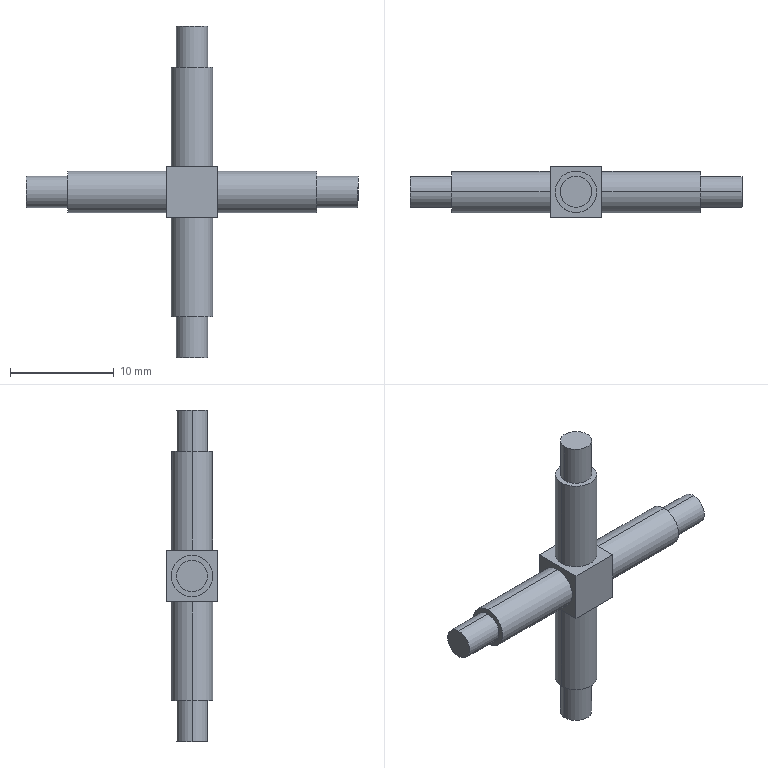Part | SolidWorks | features ICE 4, MirrorPattern 4, Extrusion 1 | 1 solid | 30 faces | box 32 x 5 x 32 mm | volume 715.619 mm3 | cylinder 16 | plane 14 | commonest cylinder face diameters 3 x8 4 x8
STEP:
#1=CARTESIAN_POINT('',(-16.194,28.299,4.));
#2=VERTEX_POINT('',#1);
#3=CARTESIAN_POINT('',(-16.194,28.299,1.));
#4=VERTEX_POINT('',#3);
#5=CARTESIAN_POINT('',(-16.194,28.299,2.5));
#6=DIRECTION('',(-1.,0.,0.));
#7=DIRECTION('',(0.,0.,1.));
#8=AXIS2_PLACEMENT_3D('',#5,#6,#7);
#9=CIRCLE('',#8,1.5);
#10=EDGE_CURVE('',#2,#4,#9,.T.);
#11=ORIENTED_EDGE('',*,*,#10,.F.);
#12=CARTESIAN_POINT('',(-12.194,28.299,4.));
#13=VERTEX_POINT('',#12);
#14=CARTESIAN_POINT('',(-16.194,28.299,4.));
#15=DIRECTION('',(1.,0.,0.));
#16=VECTOR('',#15,1000.);
#17=LINE('',#14,#16);
#18=EDGE_CURVE('',#2,#13,#17,.T.);
#19=ORIENTED_EDGE('',*,*,#18,.T.);
#20=CARTESIAN_POINT('',(-12.194,28.299,1.));
#21=VERTEX_POINT('',#20);
#22=CARTESIAN_POINT('',(-12.194,28.299,2.5));
#23=DIRECTION('',(-1.,0.,0.));
#24=DIRECTION('',(0.,0.,1.));
#25=AXIS2_PLACEMENT_3D('',#22,#23,#24);
#26=CIRCLE('',#25,1.5);
#27=EDGE_CURVE('',#13,#21,#26,.T.);
#28=ORIENTED_EDGE('',*,*,#27,.T.);
#29=CARTESIAN_POINT('',(-16.194,28.299,1.));
#30=DIRECTION('',(1.,0.,0.));
#31=VECTOR('',#30,1000.);
#32=LINE('',#29,#31);
#33=EDGE_CURVE('',#4,#21,#32,.T.);
#34=ORIENTED_EDGE('',*,*,#33,.F.);
#35=EDGE_LOOP('',(#11,#19,#28,#34));
#36=FACE_OUTER_BOUND('',#35,.T.);
#37=CARTESIAN_POINT('',(-16.194,28.299,2.5));
#38=DIRECTION('',(1.,0.,0.));
#39=DIRECTION('',(0.,0.,-1.));
#40=AXIS2_PLACEMENT_3D('',#37,#38,#39);
#41=CYLINDRICAL_SURFACE('',#40,1.5);
#42=ADVANCED_FACE('',(#36),#41,.T.);
#43=CARTESIAN_POINT('',(-40.194,28.299,4.));
#44=VERTEX_POINT('',#43);
#45=CARTESIAN_POINT('',(-40.194,28.299,1.));
#46=VERTEX_POINT('',#45);
#47=CARTESIAN_POINT('',(-40.194,28.299,2.5));
#48=DIRECTION('',(-1.,0.,0.));
#49=DIRECTION('',(0.,0.,1.));
#50=AXIS2_PLACEMENT_3D('',#47,#48,#49);
#51=CIRCLE('',#50,1.5);
#52=EDGE_CURVE('',#44,#46,#51,.T.);
#53=ORIENTED_EDGE('',*,*,#52,.T.);
#54=CARTESIAN_POINT('',(-44.194,28.299,1.));
#55=VERTEX_POINT('',#54);
#56=CARTESIAN_POINT('',(-40.194,28.299,1.));
#57=DIRECTION('',(-1.,0.,0.));
#58=VECTOR('',#57,1000.);
#59=LINE('',#56,#58);
#60=EDGE_CURVE('',#46,#55,#59,.T.);
#61=ORIENTED_EDGE('',*,*,#60,.T.);
#62=CARTESIAN_POINT('',(-44.194,28.299,4.));
#63=VERTEX_POINT('',#62);
#64=CARTESIAN_POINT('',(-44.194,28.299,2.5));
#65=DIRECTION('',(-1.,0.,0.));
#66=DIRECTION('',(0.,0.,1.));
#67=AXIS2_PLACEMENT_3D('',#64,#65,#66);
#68=CIRCLE('',#67,1.5);
#69=EDGE_CURVE('',#63,#55,#68,.T.);
#70=ORIENTED_EDGE('',*,*,#69,.F.);
#71=CARTESIAN_POINT('',(-40.194,28.299,4.));
#72=DIRECTION('',(-1.,0.,0.));
#73=VECTOR('',#72,1000.);
#74=LINE('',#71,#73);
#75=EDGE_CURVE('',#44,#63,#74,.T.);
#76=ORIENTED_EDGE('',*,*,#75,.F.);
#77=EDGE_LOOP('',(#53,#61,#70,#76));
#78=FACE_OUTER_BOUND('',#77,.T.);
#79=CARTESIAN_POINT('',(-40.194,28.299,2.5));
#80=DIRECTION('',(-1.,0.,0.));
#81=DIRECTION('',(0.,0.,1.));
#82=AXIS2_PLACEMENT_3D('',#79,#80,#81);
#83=CYLINDRICAL_SURFACE('',#82,1.5);
#84=ADVANCED_FACE('',(#78),#83,.T.);
#85=CARTESIAN_POINT('',(-26.694,28.299,-9.5));
#86=VERTEX_POINT('',#85);
#87=CARTESIAN_POINT('',(-29.694,28.299,-9.5));
#88=VERTEX_POINT('',#87);
#89=CARTESIAN_POINT('',(-28.194,28.299,-9.5));
#90=DIRECTION('',(0.,0.,1.));
#91=DIRECTION('',(1.,0.,0.));
#92=AXIS2_PLACEMENT_3D('',#89,#90,#91);
#93=CIRCLE('',#92,1.5);
#94=EDGE_CURVE('',#86,#88,#93,.T.);
#95=ORIENTED_EDGE('',*,*,#94,.F.);
#96=CARTESIAN_POINT('',(-26.694,28.299,-13.5));
#97=VERTEX_POINT('',#96);
#98=CARTESIAN_POINT('',(-26.694,28.299,-9.5));
#99=DIRECTION('',(0.,0.,-1.));
#100=VECTOR('',#99,1000.);
#101=LINE('',#98,#100);
#102=EDGE_CURVE('',#86,#97,#101,.T.);
#103=ORIENTED_EDGE('',*,*,#102,.T.);
#104=CARTESIAN_POINT('',(-29.694,28.299,-13.5));
#105=VERTEX_POINT('',#104);
#106=CARTESIAN_POINT('',(-28.194,28.299,-13.5));
#107=DIRECTION('',(0.,0.,1.));
#108=DIRECTION('',(1.,0.,0.));
#109=AXIS2_PLACEMENT_3D('',#106,#107,#108);
#110=CIRCLE('',#109,1.5);
#111=EDGE_CURVE('',#97,#105,#110,.T.);
#112=ORIENTED_EDGE('',*,*,#111,.T.);
#113=CARTESIAN_POINT('',(-29.694,28.299,-9.5));
#114=DIRECTION('',(0.,0.,-1.));
#115=VECTOR('',#114,1000.);
#116=LINE('',#113,#115);
#117=EDGE_CURVE('',#88,#105,#116,.T.);
#118=ORIENTED_EDGE('',*,*,#117,.F.);
#119=EDGE_LOOP('',(#95,#103,#112,#118));
#120=FACE_OUTER_BOUND('',#119,.T.);
#121=CARTESIAN_POINT('',(-28.194,28.299,-9.5));
#122=DIRECTION('',(0.,0.,-1.));
#123=DIRECTION('',(-1.,0.,0.));
#124=AXIS2_PLACEMENT_3D('',#121,#122,#123);
#125=CYLINDRICAL_SURFACE('',#124,1.5);
#126=ADVANCED_FACE('',(#120),#125,.T.);
#127=CARTESIAN_POINT('',(-26.694,28.299,14.5));
#128=VERTEX_POINT('',#127);
#129=CARTESIAN_POINT('',(-29.694,28.299,14.5));
#130=VERTEX_POINT('',#129);
#131=CARTESIAN_POINT('',(-28.194,28.299,14.5));
#132=DIRECTION('',(0.,0.,1.));
#133=DIRECTION('',(1.,0.,0.));
#134=AXIS2_PLACEMENT_3D('',#131,#132,#133);
#135=CIRCLE('',#134,1.5);
#136=EDGE_CURVE('',#128,#130,#135,.T.);
#137=ORIENTED_EDGE('',*,*,#136,.T.);
#138=CARTESIAN_POINT('',(-29.694,28.299,18.5));
#139=VERTEX_POINT('',#138);
#140=CARTESIAN_POINT('',(-29.694,28.299,14.5));
#141=DIRECTION('',(0.,0.,1.));
#142=VECTOR('',#141,1000.);
#143=LINE('',#140,#142);
#144=EDGE_CURVE('',#130,#139,#143,.T.);
#145=ORIENTED_EDGE('',*,*,#144,.T.);
#146=CARTESIAN_POINT('',(-26.694,28.299,18.5));
#147=VERTEX_POINT('',#146);
#148=CARTESIAN_POINT('',(-28.194,28.299,18.5));
#149=DIRECTION('',(0.,0.,1.));
#150=DIRECTION('',(1.,0.,0.));
#151=AXIS2_PLACEMENT_3D('',#148,#149,#150);
#152=CIRCLE('',#151,1.5);
#153=EDGE_CURVE('',#147,#139,#152,.T.);
#154=ORIENTED_EDGE('',*,*,#153,.F.);
#155=CARTESIAN_POINT('',(-26.694,28.299,14.5));
#156=DIRECTION('',(0.,0.,1.));
#157=VECTOR('',#156,1000.);
#158=LINE('',#155,#157);
#159=EDGE_CURVE('',#128,#147,#158,.T.);
#160=ORIENTED_EDGE('',*,*,#159,.F.);
#161=EDGE_LOOP('',(#137,#145,#154,#160));
#162=FACE_OUTER_BOUND('',#161,.T.);
#163=CARTESIAN_POINT('',(-28.194,28.299,14.5));
#164=DIRECTION('',(0.,0.,1.));
#165=DIRECTION('',(1.,0.,0.));
#166=AXIS2_PLACEMENT_3D('',#163,#164,#165);
#167=CYLINDRICAL_SURFACE('',#166,1.5);
#168=ADVANCED_FACE('',(#162),#167,.T.);
#169=CARTESIAN_POINT('',(-26.194,28.299,14.5));
#170=VERTEX_POINT('',#169);
#171=CARTESIAN_POINT('',(-30.194,28.299,14.5));
#172=VERTEX_POINT('',#171);
#173=CARTESIAN_POINT('',(-28.194,28.299,14.5));
#174=DIRECTION('',(0.,0.,1.));
#175=DIRECTION('',(1.,0.,0.));
#176=AXIS2_PLACEMENT_3D('',#173,#174,#175);
#177=CIRCLE('',#176,2.);
#178=EDGE_CURVE('',#170,#172,#177,.T.);
#179=ORIENTED_EDGE('',*,*,#178,.F.);
#180=CARTESIAN_POINT('',(-26.194,28.299,5.));
#181=VERTEX_POINT('',#180);
#182=CARTESIAN_POINT('',(-26.194,28.299,18.5));
#183=DIRECTION('',(0.,0.,-1.));
#184=VECTOR('',#183,1000.);
#185=LINE('',#182,#184);
#186=EDGE_CURVE('',#170,#181,#185,.T.);
#187=ORIENTED_EDGE('',*,*,#186,.T.);
#188=CARTESIAN_POINT('',(-30.194,28.299,5.));
#189=VERTEX_POINT('',#188);
#190=CARTESIAN_POINT('',(-28.194,28.299,5.));
#191=DIRECTION('',(0.,0.,1.));
#192=DIRECTION('',(1.,0.,0.));
#193=AXIS2_PLACEMENT_3D('',#190,#191,#192);
#194=CIRCLE('',#193,2.);
#195=EDGE_CURVE('',#181,#189,#194,.T.);
#196=ORIENTED_EDGE('',*,*,#195,.T.);
#197=CARTESIAN_POINT('',(-30.194,28.299,18.5));
#198=DIRECTION('',(0.,0.,-1.));
#199=VECTOR('',#198,1000.);
#200=LINE('',#197,#199);
#201=EDGE_CURVE('',#172,#189,#200,.T.);
#202=ORIENTED_EDGE('',*,*,#201,.F.);
#203=EDGE_LOOP('',(#179,#187,#196,#202));
#204=FACE_OUTER_BOUND('',#203,.T.);
#205=CARTESIAN_POINT('',(-28.194,28.299,18.5));
#206=DIRECTION('',(0.,0.,-1.));
#207=DIRECTION('',(-1.,0.,0.));
#208=AXIS2_PLACEMENT_3D('',#205,#206,#207);
#209=CYLINDRICAL_SURFACE('',#208,2.);
#210=ADVANCED_FACE('',(#204),#209,.T.);
#211=CARTESIAN_POINT('',(-26.194,28.299,-9.5));
#212=VERTEX_POINT('',#211);
#213=CARTESIAN_POINT('',(-30.194,28.299,-9.5));
#214=VERTEX_POINT('',#213);
#215=CARTESIAN_POINT('',(-28.194,28.299,-9.5));
#216=DIRECTION('',(0.,0.,1.));
#217=DIRECTION('',(1.,0.,0.));
#218=AXIS2_PLACEMENT_3D('',#215,#216,#217);
#219=CIRCLE('',#218,2.);
#220=EDGE_CURVE('',#212,#214,#219,.T.);
#221=ORIENTED_EDGE('',*,*,#220,.T.);
#222=CARTESIAN_POINT('',(-30.194,28.299,0.));
#223=VERTEX_POINT('',#222);
#224=CARTESIAN_POINT('',(-30.194,28.299,-13.5));
#225=DIRECTION('',(0.,0.,1.));
#226=VECTOR('',#225,1000.);
#227=LINE('',#224,#226);
#228=EDGE_CURVE('',#214,#223,#227,.T.);
#229=ORIENTED_EDGE('',*,*,#228,.T.);
#230=CARTESIAN_POINT('',(-26.194,28.299,0.));
#231=VERTEX_POINT('',#230);
#232=CARTESIAN_POINT('',(-28.194,28.299,0.));
#233=DIRECTION('',(0.,0.,1.));
#234=DIRECTION('',(1.,0.,0.));
#235=AXIS2_PLACEMENT_3D('',#232,#233,#234);
#236=CIRCLE('',#235,2.);
#237=EDGE_CURVE('',#231,#223,#236,.T.);
#238=ORIENTED_EDGE('',*,*,#237,.F.);
#239=CARTESIAN_POINT('',(-26.194,28.299,-13.5));
#240=DIRECTION('',(0.,0.,1.));
#241=VECTOR('',#240,1000.);
#242=LINE('',#239,#241);
#243=EDGE_CURVE('',#212,#231,#242,.T.);
#244=ORIENTED_EDGE('',*,*,#243,.F.);
#245=EDGE_LOOP('',(#221,#229,#238,#244));
#246=FACE_OUTER_BOUND('',#245,.T.);
#247=CARTESIAN_POINT('',(-28.194,28.299,-13.5));
#248=DIRECTION('',(0.,0.,1.));
#249=DIRECTION('',(1.,0.,0.));
#250=AXIS2_PLACEMENT_3D('',#247,#248,#249);
#251=CYLINDRICAL_SURFACE('',#250,2.);
#252=ADVANCED_FACE('',(#246),#251,.T.);
#253=CARTESIAN_POINT('',(-40.194,28.299,4.5));
#254=VERTEX_POINT('',#253);
#255=CARTESIAN_POINT('',(-40.194,28.299,0.5));
#256=VERTEX_POINT('',#255);
#257=CARTESIAN_POINT('',(-40.194,28.299,2.5));
#258=DIRECTION('',(-1.,0.,0.));
#259=DIRECTION('',(0.,0.,1.));
#260=AXIS2_PLACEMENT_3D('',#257,#258,#259);
#261=CIRCLE('',#260,2.);
#262=EDGE_CURVE('',#254,#256,#261,.T.);
#263=ORIENTED_EDGE('',*,*,#262,.F.);
#264=CARTESIAN_POINT('',(-30.694,28.299,4.5));
#265=VERTEX_POINT('',#264);
#266=CARTESIAN_POINT('',(-44.194,28.299,4.5));
#267=DIRECTION('',(1.,0.,0.));
#268=VECTOR('',#267,1000.);
#269=LINE('',#266,#268);
#270=EDGE_CURVE('',#254,#265,#269,.T.);
#271=ORIENTED_EDGE('',*,*,#270,.T.);
#272=CARTESIAN_POINT('',(-30.694,28.299,0.5));
#273=VERTEX_POINT('',#272);
#274=CARTESIAN_POINT('',(-30.694,28.299,2.5));
#275=DIRECTION('',(1.,0.,0.));
#276=DIRECTION('',(0.,0.,-1.));
#277=AXIS2_PLACEMENT_3D('',#274,#275,#276);
#278=CIRCLE('',#277,2.);
#279=EDGE_CURVE('',#273,#265,#278,.T.);
#280=ORIENTED_EDGE('',*,*,#279,.F.);
#281=CARTESIAN_POINT('',(-44.194,28.299,0.5));
#282=DIRECTION('',(1.,0.,0.));
#283=VECTOR('',#282,1000.);
#284=LINE('',#281,#283);
#285=EDGE_CURVE('',#256,#273,#284,.T.);
#286=ORIENTED_EDGE('',*,*,#285,.F.);
#287=EDGE_LOOP('',(#263,#271,#280,#286));
#288=FACE_OUTER_BOUND('',#287,.T.);
#289=CARTESIAN_POINT('',(-44.194,28.299,2.5));
#290=DIRECTION('',(1.,0.,0.));
#291=DIRECTION('',(0.,0.,-1.));
#292=AXIS2_PLACEMENT_3D('',#289,#290,#291);
#293=CYLINDRICAL_SURFACE('',#292,2.);
#294=ADVANCED_FACE('',(#288),#293,.T.);
#295=CARTESIAN_POINT('',(-16.194,28.299,4.5));
#296=VERTEX_POINT('',#295);
#297=CARTESIAN_POINT('',(-16.194,28.299,0.5));
#298=VERTEX_POINT('',#297);
#299=CARTESIAN_POINT('',(-16.194,28.299,2.5));
#300=DIRECTION('',(-1.,0.,0.));
#301=DIRECTION('',(0.,0.,1.));
#302=AXIS2_PLACEMENT_3D('',#299,#300,#301);
#303=CIRCLE('',#302,2.);
#304=EDGE_CURVE('',#296,#298,#303,.T.);
#305=ORIENTED_EDGE('',*,*,#304,.T.);
#306=CARTESIAN_POINT('',(-25.694,28.299,0.5));
#307=VERTEX_POINT('',#306);
#308=CARTESIAN_POINT('',(-12.194,28.299,0.5));
#309=DIRECTION('',(-1.,0.,0.));
#310=VECTOR('',#309,1000.);
#311=LINE('',#308,#310);
#312=EDGE_CURVE('',#298,#307,#311,.T.);
#313=ORIENTED_EDGE('',*,*,#312,.T.);
#314=CARTESIAN_POINT('',(-25.694,28.299,4.5));
#315=VERTEX_POINT('',#314);
#316=CARTESIAN_POINT('',(-25.694,28.299,2.5));
#317=DIRECTION('',(1.,0.,0.));
#318=DIRECTION('',(0.,0.,-1.));
#319=AXIS2_PLACEMENT_3D('',#316,#317,#318);
#320=CIRCLE('',#319,2.);
#321=EDGE_CURVE('',#307,#315,#320,.T.);
#322=ORIENTED_EDGE('',*,*,#321,.T.);
#323=CARTESIAN_POINT('',(-12.194,28.299,4.5));
#324=DIRECTION('',(-1.,0.,0.));
#325=VECTOR('',#324,1000.);
#326=LINE('',#323,#325);
#327=EDGE_CURVE('',#296,#315,#326,.T.);
#328=ORIENTED_EDGE('',*,*,#327,.F.);
#329=EDGE_LOOP('',(#305,#313,#322,#328));
#330=FACE_OUTER_BOUND('',#329,.T.);
#331=CARTESIAN_POINT('',(-12.194,28.299,2.5));
#332=DIRECTION('',(-1.,0.,0.));
#333=DIRECTION('',(0.,0.,1.));
#334=AXIS2_PLACEMENT_3D('',#331,#332,#333);
#335=CYLINDRICAL_SURFACE('',#334,2.);
#336=ADVANCED_FACE('',(#330),#335,.T.);
#337=ORIENTED_EDGE('',*,*,#312,.F.);
#338=CARTESIAN_POINT('',(-16.194,28.299,2.5));
#339=DIRECTION('',(-1.,0.,0.));
#340=DIRECTION('',(0.,0.,1.));
#341=AXIS2_PLACEMENT_3D('',#338,#339,#340);
#342=CIRCLE('',#341,2.);
#343=EDGE_CURVE('',#298,#296,#342,.T.);
#344=ORIENTED_EDGE('',*,*,#343,.T.);
#345=ORIENTED_EDGE('',*,*,#327,.T.);
#346=CARTESIAN_POINT('',(-25.694,28.299,2.5));
#347=DIRECTION('',(1.,0.,0.));
#348=DIRECTION('',(0.,0.,-1.));
#349=AXIS2_PLACEMENT_3D('',#346,#347,#348);
#350=CIRCLE('',#349,2.);
#351=EDGE_CURVE('',#315,#307,#350,.T.);
#352=ORIENTED_EDGE('',*,*,#351,.T.);
#353=EDGE_LOOP('',(#337,#344,#345,#352));
#354=FACE_OUTER_BOUND('',#353,.T.);
#355=CARTESIAN_POINT('',(-12.194,28.299,2.5));
#356=DIRECTION('',(-1.,0.,0.));
#357=DIRECTION('',(0.,0.,1.));
#358=AXIS2_PLACEMENT_3D('',#355,#356,#357);
#359=CYLINDRICAL_SURFACE('',#358,2.);
#360=ADVANCED_FACE('',(#354),#359,.T.);
#361=ORIENTED_EDGE('',*,*,#270,.F.);
#362=CARTESIAN_POINT('',(-40.194,28.299,2.5));
#363=DIRECTION('',(-1.,0.,0.));
#364=DIRECTION('',(0.,0.,1.));
#365=AXIS2_PLACEMENT_3D('',#362,#363,#364);
#366=CIRCLE('',#365,2.);
#367=EDGE_CURVE('',#256,#254,#366,.T.);
#368=ORIENTED_EDGE('',*,*,#367,.F.);
#369=ORIENTED_EDGE('',*,*,#285,.T.);
#370=CARTESIAN_POINT('',(-30.694,28.299,2.5));
#371=DIRECTION('',(1.,0.,0.));
#372=DIRECTION('',(0.,0.,-1.));
#373=AXIS2_PLACEMENT_3D('',#370,#371,#372);
#374=CIRCLE('',#373,2.);
#375=EDGE_CURVE('',#265,#273,#374,.T.);
#376=ORIENTED_EDGE('',*,*,#375,.F.);
#377=EDGE_LOOP('',(#361,#368,#369,#376));
#378=FACE_OUTER_BOUND('',#377,.T.);
#379=CARTESIAN_POINT('',(-44.194,28.299,2.5));
#380=DIRECTION('',(1.,0.,0.));
#381=DIRECTION('',(0.,0.,-1.));
#382=AXIS2_PLACEMENT_3D('',#379,#380,#381);
#383=CYLINDRICAL_SURFACE('',#382,2.);
#384=ADVANCED_FACE('',(#378),#383,.T.);
#385=ORIENTED_EDGE('',*,*,#228,.F.);
#386=CARTESIAN_POINT('',(-28.194,28.299,-9.5));
#387=DIRECTION('',(0.,0.,1.));
#388=DIRECTION('',(1.,0.,0.));
#389=AXIS2_PLACEMENT_3D('',#386,#387,#388);
#390=CIRCLE('',#389,2.);
#391=EDGE_CURVE('',#214,#212,#390,.T.);
#392=ORIENTED_EDGE('',*,*,#391,.T.);
#393=ORIENTED_EDGE('',*,*,#243,.T.);
#394=CARTESIAN_POINT('',(-28.194,28.299,0.));
#395=DIRECTION('',(0.,0.,1.));
#396=DIRECTION('',(1.,0.,0.));
#397=AXIS2_PLACEMENT_3D('',#394,#395,#396);
#398=CIRCLE('',#397,2.);
#399=EDGE_CURVE('',#223,#231,#398,.T.);
#400=ORIENTED_EDGE('',*,*,#399,.F.);
#401=EDGE_LOOP('',(#385,#392,#393,#400));
#402=FACE_OUTER_BOUND('',#401,.T.);
#403=CARTESIAN_POINT('',(-28.194,28.299,-13.5));
#404=DIRECTION('',(0.,0.,1.));
#405=DIRECTION('',(1.,0.,0.));
#406=AXIS2_PLACEMENT_3D('',#403,#404,#405);
#407=CYLINDRICAL_SURFACE('',#406,2.);
#408=ADVANCED_FACE('',(#402),#407,.T.);
#409=ORIENTED_EDGE('',*,*,#186,.F.);
#410=CARTESIAN_POINT('',(-28.194,28.299,14.5));
#411=DIRECTION('',(0.,0.,1.));
#412=DIRECTION('',(1.,0.,0.));
#413=AXIS2_PLACEMENT_3D('',#410,#411,#412);
#414=CIRCLE('',#413,2.);
#415=EDGE_CURVE('',#172,#170,#414,.T.);
#416=ORIENTED_EDGE('',*,*,#415,.F.);
#417=ORIENTED_EDGE('',*,*,#201,.T.);
#418=CARTESIAN_POINT('',(-28.194,28.299,5.));
#419=DIRECTION('',(0.,0.,1.));
#420=DIRECTION('',(1.,0.,0.));
#421=AXIS2_PLACEMENT_3D('',#418,#419,#420);
#422=CIRCLE('',#421,2.);
#423=EDGE_CURVE('',#189,#181,#422,.T.);
#424=ORIENTED_EDGE('',*,*,#423,.T.);
#425=EDGE_LOOP('',(#409,#416,#417,#424));
#426=FACE_OUTER_BOUND('',#425,.T.);
#427=CARTESIAN_POINT('',(-28.194,28.299,18.5));
#428=DIRECTION('',(0.,0.,-1.));
#429=DIRECTION('',(-1.,0.,0.));
#430=AXIS2_PLACEMENT_3D('',#427,#428,#429);
#431=CYLINDRICAL_SURFACE('',#430,2.);
#432=ADVANCED_FACE('',(#426),#431,.T.);
#433=ORIENTED_EDGE('',*,*,#279,.T.);
#434=ORIENTED_EDGE('',*,*,#375,.T.);
#435=EDGE_LOOP('',(#433,#434));
#436=FACE_BOUND('',#435,.T.);
#437=CARTESIAN_POINT('',(-30.694,30.799,0.));
#438=VERTEX_POINT('',#437);
#439=CARTESIAN_POINT('',(-30.694,25.799,0.));
#440=VERTEX_POINT('',#439);
#441=CARTESIAN_POINT('',(-30.694,25.799,0.));
#442=DIRECTION('',(0.,-1.,0.));
#443=VECTOR('',#442,1000.);
#444=LINE('',#441,#443);
#445=EDGE_CURVE('',#438,#440,#444,.T.);
#446=ORIENTED_EDGE('',*,*,#445,.T.);
#447=CARTESIAN_POINT('',(-30.694,25.799,5.));
#448=VERTEX_POINT('',#447);
#449=CARTESIAN_POINT('',(-30.694,25.799,5.));
#450=DIRECTION('',(0.,0.,-1.));
#451=VECTOR('',#450,1000.);
#452=LINE('',#449,#451);
#453=EDGE_CURVE('',#448,#440,#452,.T.);
#454=ORIENTED_EDGE('',*,*,#453,.F.);
#455=CARTESIAN_POINT('',(-30.694,30.799,5.));
#456=VERTEX_POINT('',#455);
#457=CARTESIAN_POINT('',(-30.694,25.799,5.));
#458=DIRECTION('',(0.,-1.,0.));
#459=VECTOR('',#458,1000.);
#460=LINE('',#457,#459);
#461=EDGE_CURVE('',#456,#448,#460,.T.);
#462=ORIENTED_EDGE('',*,*,#461,.F.);
#463=CARTESIAN_POINT('',(-30.694,30.799,5.));
#464=DIRECTION('',(0.,0.,-1.));
#465=VECTOR('',#464,1000.);
#466=LINE('',#463,#465);
#467=EDGE_CURVE('',#456,#438,#466,.T.);
#468=ORIENTED_EDGE('',*,*,#467,.T.);
#469=EDGE_LOOP('',(#446,#454,#462,#468));
#470=FACE_OUTER_BOUND('',#469,.T.);
#471=CARTESIAN_POINT('',(-30.694,25.799,5.));
#472=DIRECTION('',(1.,0.,0.));
#473=DIRECTION('',(0.,0.,-1.));
#474=AXIS2_PLACEMENT_3D('',#471,#472,#473);
#475=PLANE('',#474);
#476=ADVANCED_FACE('',(#436,#470),#475,.F.);
#477=CARTESIAN_POINT('',(-25.694,25.799,0.));
#478=VERTEX_POINT('',#477);
#479=CARTESIAN_POINT('',(-25.694,25.799,0.));
#480=DIRECTION('',(1.,0.,0.));
#481=VECTOR('',#480,1000.);
#482=LINE('',#479,#481);
#483=EDGE_CURVE('',#440,#478,#482,.T.);
#484=ORIENTED_EDGE('',*,*,#483,.T.);
#485=CARTESIAN_POINT('',(-25.694,25.799,5.));
#486=VERTEX_POINT('',#485);
#487=CARTESIAN_POINT('',(-25.694,25.799,5.));
#488=DIRECTION('',(0.,0.,-1.));
#489=VECTOR('',#488,1000.);
#490=LINE('',#487,#489);
#491=EDGE_CURVE('',#486,#478,#490,.T.);
#492=ORIENTED_EDGE('',*,*,#491,.F.);
#493=CARTESIAN_POINT('',(-25.694,25.799,5.));
#494=DIRECTION('',(1.,0.,0.));
#495=VECTOR('',#494,1000.);
#496=LINE('',#493,#495);
#497=EDGE_CURVE('',#448,#486,#496,.T.);
#498=ORIENTED_EDGE('',*,*,#497,.F.);
#499=ORIENTED_EDGE('',*,*,#453,.T.);
#500=EDGE_LOOP('',(#484,#492,#498,#499));
#501=FACE_OUTER_BOUND('',#500,.T.);
#502=CARTESIAN_POINT('',(-25.694,25.799,5.));
#503=DIRECTION('',(0.,1.,0.));
#504=DIRECTION('',(0.,0.,1.));
#505=AXIS2_PLACEMENT_3D('',#502,#503,#504);
#506=PLANE('',#505);
#507=ADVANCED_FACE('',(#501),#506,.F.);
#508=ORIENTED_EDGE('',*,*,#351,.F.);
#509=ORIENTED_EDGE('',*,*,#321,.F.);
#510=EDGE_LOOP('',(#508,#509));
#511=FACE_BOUND('',#510,.T.);
#512=CARTESIAN_POINT('',(-25.694,30.799,0.));
#513=VERTEX_POINT('',#512);
#514=CARTESIAN_POINT('',(-25.694,30.799,0.));
#515=DIRECTION('',(0.,1.,0.));
#516=VECTOR('',#515,1000.);
#517=LINE('',#514,#516);
#518=EDGE_CURVE('',#478,#513,#517,.T.);
#519=ORIENTED_EDGE('',*,*,#518,.T.);
#520=CARTESIAN_POINT('',(-25.694,30.799,5.));
#521=VERTEX_POINT('',#520);
#522=CARTESIAN_POINT('',(-25.694,30.799,5.));
#523=DIRECTION('',(0.,0.,-1.));
#524=VECTOR('',#523,1000.);
#525=LINE('',#522,#524);
#526=EDGE_CURVE('',#521,#513,#525,.T.);
#527=ORIENTED_EDGE('',*,*,#526,.F.);
#528=CARTESIAN_POINT('',(-25.694,30.799,5.));
#529=DIRECTION('',(0.,1.,0.));
#530=VECTOR('',#529,1000.);
#531=LINE('',#528,#530);
#532=EDGE_CURVE('',#486,#521,#531,.T.);
#533=ORIENTED_EDGE('',*,*,#532,.F.);
#534=ORIENTED_EDGE('',*,*,#491,.T.);
#535=EDGE_LOOP('',(#519,#527,#533,#534));
#536=FACE_OUTER_BOUND('',#535,.T.);
#537=CARTESIAN_POINT('',(-25.694,30.799,5.));
#538=DIRECTION('',(-1.,0.,0.));
#539=DIRECTION('',(0.,0.,1.));
#540=AXIS2_PLACEMENT_3D('',#537,#538,#539);
#541=PLANE('',#540);
#542=ADVANCED_FACE('',(#511,#536),#541,.F.);
#543=CARTESIAN_POINT('',(-30.694,30.799,0.));
#544=DIRECTION('',(-1.,0.,0.));
#545=VECTOR('',#544,1000.);
#546=LINE('',#543,#545);
#547=EDGE_CURVE('',#513,#438,#546,.T.);
#548=ORIENTED_EDGE('',*,*,#547,.T.);
#549=ORIENTED_EDGE('',*,*,#467,.F.);
#550=CARTESIAN_POINT('',(-30.694,30.799,5.));
#551=DIRECTION('',(-1.,0.,0.));
#552=VECTOR('',#551,1000.);
#553=LINE('',#550,#552);
#554=EDGE_CURVE('',#521,#456,#553,.T.);
#555=ORIENTED_EDGE('',*,*,#554,.F.);
#556=ORIENTED_EDGE('',*,*,#526,.T.);
#557=EDGE_LOOP('',(#548,#549,#555,#556));
#558=FACE_OUTER_BOUND('',#557,.T.);
#559=CARTESIAN_POINT('',(-30.694,30.799,5.));
#560=DIRECTION('',(0.,-1.,0.));
#561=DIRECTION('',(0.,0.,-1.));
#562=AXIS2_PLACEMENT_3D('',#559,#560,#561);
#563=PLANE('',#562);
#564=ADVANCED_FACE('',(#558),#563,.F.);
#565=ORIENTED_EDGE('',*,*,#423,.F.);
#566=ORIENTED_EDGE('',*,*,#195,.F.);
#567=EDGE_LOOP('',(#565,#566));
#568=FACE_BOUND('',#567,.T.);
#569=ORIENTED_EDGE('',*,*,#461,.T.);
#570=ORIENTED_EDGE('',*,*,#497,.T.);
#571=ORIENTED_EDGE('',*,*,#532,.T.);
#572=ORIENTED_EDGE('',*,*,#554,.T.);
#573=EDGE_LOOP('',(#569,#570,#571,#572));
#574=FACE_OUTER_BOUND('',#573,.T.);
#575=CARTESIAN_POINT('',(0.,0.,5.));
#576=DIRECTION('',(0.,0.,-1.));
#577=DIRECTION('',(-1.,0.,0.));
#578=AXIS2_PLACEMENT_3D('',#575,#576,#577);
#579=PLANE('',#578);
#580=ADVANCED_FACE('',(#568,#574),#579,.F.);
#581=ORIENTED_EDGE('',*,*,#237,.T.);
#582=ORIENTED_EDGE('',*,*,#399,.T.);
#583=EDGE_LOOP('',(#581,#582));
#584=FACE_BOUND('',#583,.T.);
#585=ORIENTED_EDGE('',*,*,#445,.F.);
#586=ORIENTED_EDGE('',*,*,#547,.F.);
#587=ORIENTED_EDGE('',*,*,#518,.F.);
#588=ORIENTED_EDGE('',*,*,#483,.F.);
#589=EDGE_LOOP('',(#585,#586,#587,#588));
#590=FACE_OUTER_BOUND('',#589,.T.);
#591=CARTESIAN_POINT('',(0.,0.,0.));
#592=DIRECTION('',(0.,0.,-1.));
#593=DIRECTION('',(-1.,0.,0.));
#594=AXIS2_PLACEMENT_3D('',#591,#592,#593);
#595=PLANE('',#594);
#596=ADVANCED_FACE('',(#584,#590),#595,.T.);
#597=ORIENTED_EDGE('',*,*,#136,.F.);
#598=CARTESIAN_POINT('',(-28.194,28.299,14.5));
#599=DIRECTION('',(0.,0.,1.));
#600=DIRECTION('',(1.,0.,0.));
#601=AXIS2_PLACEMENT_3D('',#598,#599,#600);
#602=CIRCLE('',#601,1.5);
#603=EDGE_CURVE('',#130,#128,#602,.T.);
#604=ORIENTED_EDGE('',*,*,#603,.F.);
#605=EDGE_LOOP('',(#597,#604));
#606=FACE_BOUND('',#605,.T.);
#607=ORIENTED_EDGE('',*,*,#415,.T.);
#608=ORIENTED_EDGE('',*,*,#178,.T.);
#609=EDGE_LOOP('',(#607,#608));
#610=FACE_OUTER_BOUND('',#609,.T.);
#611=CARTESIAN_POINT('',(-28.194,28.299,14.5));
#612=DIRECTION('',(0.,0.,1.));
#613=DIRECTION('',(1.,0.,0.));
#614=AXIS2_PLACEMENT_3D('',#611,#612,#613);
#615=PLANE('',#614);
#616=ADVANCED_FACE('',(#606,#610),#615,.T.);
#617=ORIENTED_EDGE('',*,*,#144,.F.);
#618=ORIENTED_EDGE('',*,*,#603,.T.);
#619=ORIENTED_EDGE('',*,*,#159,.T.);
#620=CARTESIAN_POINT('',(-28.194,28.299,18.5));
#621=DIRECTION('',(0.,0.,1.));
#622=DIRECTION('',(1.,0.,0.));
#623=AXIS2_PLACEMENT_3D('',#620,#621,#622);
#624=CIRCLE('',#623,1.5);
#625=EDGE_CURVE('',#139,#147,#624,.T.);
#626=ORIENTED_EDGE('',*,*,#625,.F.);
#627=EDGE_LOOP('',(#617,#618,#619,#626));
#628=FACE_OUTER_BOUND('',#627,.T.);
#629=CARTESIAN_POINT('',(-28.194,28.299,14.5));
#630=DIRECTION('',(0.,0.,1.));
#631=DIRECTION('',(1.,0.,0.));
#632=AXIS2_PLACEMENT_3D('',#629,#630,#631);
#633=CYLINDRICAL_SURFACE('',#632,1.5);
#634=ADVANCED_FACE('',(#628),#633,.T.);
#635=ORIENTED_EDGE('',*,*,#153,.T.);
#636=ORIENTED_EDGE('',*,*,#625,.T.);
#637=EDGE_LOOP('',(#635,#636));
#638=FACE_OUTER_BOUND('',#637,.T.);
#639=CARTESIAN_POINT('',(-28.194,28.299,18.5));
#640=DIRECTION('',(0.,0.,1.));
#641=DIRECTION('',(1.,0.,0.));
#642=AXIS2_PLACEMENT_3D('',#639,#640,#641);
#643=PLANE('',#642);
#644=ADVANCED_FACE('',(#638),#643,.T.);
#645=ORIENTED_EDGE('',*,*,#220,.F.);
#646=ORIENTED_EDGE('',*,*,#391,.F.);
#647=EDGE_LOOP('',(#645,#646));
#648=FACE_OUTER_BOUND('',#647,.T.);
#649=CARTESIAN_POINT('',(-28.194,28.299,-9.5));
#650=DIRECTION('',(0.,0.,1.));
#651=DIRECTION('',(1.,0.,0.));
#652=AXIS2_PLACEMENT_3D('',#649,#650,#651);
#653=CIRCLE('',#652,1.5);
#654=EDGE_CURVE('',#88,#86,#653,.T.);
#655=ORIENTED_EDGE('',*,*,#654,.T.);
#656=ORIENTED_EDGE('',*,*,#94,.T.);
#657=EDGE_LOOP('',(#655,#656));
#658=FACE_BOUND('',#657,.T.);
#659=CARTESIAN_POINT('',(-28.194,28.299,-9.5));
#660=DIRECTION('',(0.,0.,-1.));
#661=DIRECTION('',(1.,0.,0.));
#662=AXIS2_PLACEMENT_3D('',#659,#660,#661);
#663=PLANE('',#662);
#664=ADVANCED_FACE('',(#648,#658),#663,.T.);
#665=ORIENTED_EDGE('',*,*,#102,.F.);
#666=ORIENTED_EDGE('',*,*,#654,.F.);
#667=ORIENTED_EDGE('',*,*,#117,.T.);
#668=CARTESIAN_POINT('',(-28.194,28.299,-13.5));
#669=DIRECTION('',(0.,0.,1.));
#670=DIRECTION('',(1.,0.,0.));
#671=AXIS2_PLACEMENT_3D('',#668,#669,#670);
#672=CIRCLE('',#671,1.5);
#673=EDGE_CURVE('',#105,#97,#672,.T.);
#674=ORIENTED_EDGE('',*,*,#673,.T.);
#675=EDGE_LOOP('',(#665,#666,#667,#674));
#676=FACE_OUTER_BOUND('',#675,.T.);
#677=CARTESIAN_POINT('',(-28.194,28.299,-9.5));
#678=DIRECTION('',(0.,0.,-1.));
#679=DIRECTION('',(-1.,0.,0.));
#680=AXIS2_PLACEMENT_3D('',#677,#678,#679);
#681=CYLINDRICAL_SURFACE('',#680,1.5);
#682=ADVANCED_FACE('',(#676),#681,.T.);
#683=ORIENTED_EDGE('',*,*,#673,.F.);
#684=ORIENTED_EDGE('',*,*,#111,.F.);
#685=EDGE_LOOP('',(#683,#684));
#686=FACE_OUTER_BOUND('',#685,.T.);
#687=CARTESIAN_POINT('',(-28.194,28.299,-13.5));
#688=DIRECTION('',(0.,0.,-1.));
#689=DIRECTION('',(1.,0.,0.));
#690=AXIS2_PLACEMENT_3D('',#687,#688,#689);
#691=PLANE('',#690);
#692=ADVANCED_FACE('',(#686),#691,.T.);
#693=ORIENTED_EDGE('',*,*,#52,.F.);
#694=CARTESIAN_POINT('',(-40.194,28.299,2.5));
#695=DIRECTION('',(-1.,0.,0.));
#696=DIRECTION('',(0.,0.,1.));
#697=AXIS2_PLACEMENT_3D('',#694,#695,#696);
#698=CIRCLE('',#697,1.5);
#699=EDGE_CURVE('',#46,#44,#698,.T.);
#700=ORIENTED_EDGE('',*,*,#699,.F.);
#701=EDGE_LOOP('',(#693,#700));
#702=FACE_BOUND('',#701,.T.);
#703=ORIENTED_EDGE('',*,*,#367,.T.);
#704=ORIENTED_EDGE('',*,*,#262,.T.);
#705=EDGE_LOOP('',(#703,#704));
#706=FACE_OUTER_BOUND('',#705,.T.);
#707=CARTESIAN_POINT('',(-40.194,28.299,2.5));
#708=DIRECTION('',(-1.,0.,0.));
#709=DIRECTION('',(0.,0.,1.));
#710=AXIS2_PLACEMENT_3D('',#707,#708,#709);
#711=PLANE('',#710);
#712=ADVANCED_FACE('',(#702,#706),#711,.T.);
#713=ORIENTED_EDGE('',*,*,#60,.F.);
#714=ORIENTED_EDGE('',*,*,#699,.T.);
#715=ORIENTED_EDGE('',*,*,#75,.T.);
#716=CARTESIAN_POINT('',(-44.194,28.299,2.5));
#717=DIRECTION('',(-1.,0.,0.));
#718=DIRECTION('',(0.,0.,1.));
#719=AXIS2_PLACEMENT_3D('',#716,#717,#718);
#720=CIRCLE('',#719,1.5);
#721=EDGE_CURVE('',#55,#63,#720,.T.);
#722=ORIENTED_EDGE('',*,*,#721,.F.);
#723=EDGE_LOOP('',(#713,#714,#715,#722));
#724=FACE_OUTER_BOUND('',#723,.T.);
#725=CARTESIAN_POINT('',(-40.194,28.299,2.5));
#726=DIRECTION('',(-1.,0.,0.));
#727=DIRECTION('',(0.,0.,1.));
#728=AXIS2_PLACEMENT_3D('',#725,#726,#727);
#729=CYLINDRICAL_SURFACE('',#728,1.5);
#730=ADVANCED_FACE('',(#724),#729,.T.);
#731=ORIENTED_EDGE('',*,*,#69,.T.);
#732=ORIENTED_EDGE('',*,*,#721,.T.);
#733=EDGE_LOOP('',(#731,#732));
#734=FACE_OUTER_BOUND('',#733,.T.);
#735=CARTESIAN_POINT('',(-44.194,28.299,2.5));
#736=DIRECTION('',(-1.,0.,0.));
#737=DIRECTION('',(0.,0.,-1.));
#738=AXIS2_PLACEMENT_3D('',#735,#736,#737);
#739=PLANE('',#738);
#740=ADVANCED_FACE('',(#734),#739,.T.);
#741=ORIENTED_EDGE('',*,*,#304,.F.);
#742=ORIENTED_EDGE('',*,*,#343,.F.);
#743=EDGE_LOOP('',(#741,#742));
#744=FACE_OUTER_BOUND('',#743,.T.);
#745=CARTESIAN_POINT('',(-16.194,28.299,2.5));
#746=DIRECTION('',(-1.,0.,0.));
#747=DIRECTION('',(0.,0.,1.));
#748=AXIS2_PLACEMENT_3D('',#745,#746,#747);
#749=CIRCLE('',#748,1.5);
#750=EDGE_CURVE('',#4,#2,#749,.T.);
#751=ORIENTED_EDGE('',*,*,#750,.T.);
#752=ORIENTED_EDGE('',*,*,#10,.T.);
#753=EDGE_LOOP('',(#751,#752));
#754=FACE_BOUND('',#753,.T.);
#755=CARTESIAN_POINT('',(-16.194,28.299,2.5));
#756=DIRECTION('',(1.,0.,0.));
#757=DIRECTION('',(0.,0.,1.));
#758=AXIS2_PLACEMENT_3D('',#755,#756,#757);
#759=PLANE('',#758);
#760=ADVANCED_FACE('',(#744,#754),#759,.T.);
#761=ORIENTED_EDGE('',*,*,#18,.F.);
#762=ORIENTED_EDGE('',*,*,#750,.F.);
#763=ORIENTED_EDGE('',*,*,#33,.T.);
#764=CARTESIAN_POINT('',(-12.194,28.299,2.5));
#765=DIRECTION('',(-1.,0.,0.));
#766=DIRECTION('',(0.,0.,1.));
#767=AXIS2_PLACEMENT_3D('',#764,#765,#766);
#768=CIRCLE('',#767,1.5);
#769=EDGE_CURVE('',#21,#13,#768,.T.);
#770=ORIENTED_EDGE('',*,*,#769,.T.);
#771=EDGE_LOOP('',(#761,#762,#763,#770));
#772=FACE_OUTER_BOUND('',#771,.T.);
#773=CARTESIAN_POINT('',(-16.194,28.299,2.5));
#774=DIRECTION('',(1.,0.,0.));
#775=DIRECTION('',(0.,0.,-1.));
#776=AXIS2_PLACEMENT_3D('',#773,#774,#775);
#777=CYLINDRICAL_SURFACE('',#776,1.5);
#778=ADVANCED_FACE('',(#772),#777,.T.);
#779=ORIENTED_EDGE('',*,*,#769,.F.);
#780=ORIENTED_EDGE('',*,*,#27,.F.);
#781=EDGE_LOOP('',(#779,#780));
#782=FACE_OUTER_BOUND('',#781,.T.);
#783=CARTESIAN_POINT('',(-12.194,28.299,2.5));
#784=DIRECTION('',(1.,0.,0.));
#785=DIRECTION('',(0.,0.,-1.));
#786=AXIS2_PLACEMENT_3D('',#783,#784,#785);
#787=PLANE('',#786);
#788=ADVANCED_FACE('',(#782),#787,.T.);
#789=CLOSED_SHELL('',(#42,#84,#126,#168,#210,#252,#294,#336,#360,#384,#408,#432,#476,#507,#542,#564,#580,#596,#616,#634,#644,#664,#682,#692,#712,#730,#740,#760,#778,#788));
#790=MANIFOLD_SOLID_BREP('',#789);
#791=CARTESIAN_POINT('',(0.,0.,0.));
#792=DIRECTION('',(0.,0.,1.));
#793=DIRECTION('',(1.,0.,0.));
#794=AXIS2_PLACEMENT_3D('',#791,#792,#793);
#795=(LENGTH_UNIT()NAMED_UNIT(*)SI_UNIT(.MILLI.,.METRE.));
#796=UNCERTAINTY_MEASURE_WITH_UNIT(LENGTH_MEASURE(0.00001),#795,'','');
#797=(NAMED_UNIT(*)PLANE_ANGLE_UNIT()SI_UNIT($,.RADIAN.));
#798=(NAMED_UNIT(*)SI_UNIT($,.STERADIAN.)SOLID_ANGLE_UNIT());
#799=(GEOMETRIC_REPRESENTATION_CONTEXT(3)GLOBAL_UNCERTAINTY_ASSIGNED_CONTEXT((#796))GLOBAL_UNIT_ASSIGNED_CONTEXT((#795,#797,#798))REPRESENTATION_CONTEXT('',''));
#800=ADVANCED_BREP_SHAPE_REPRESENTATION('',(#790,#794),#799);